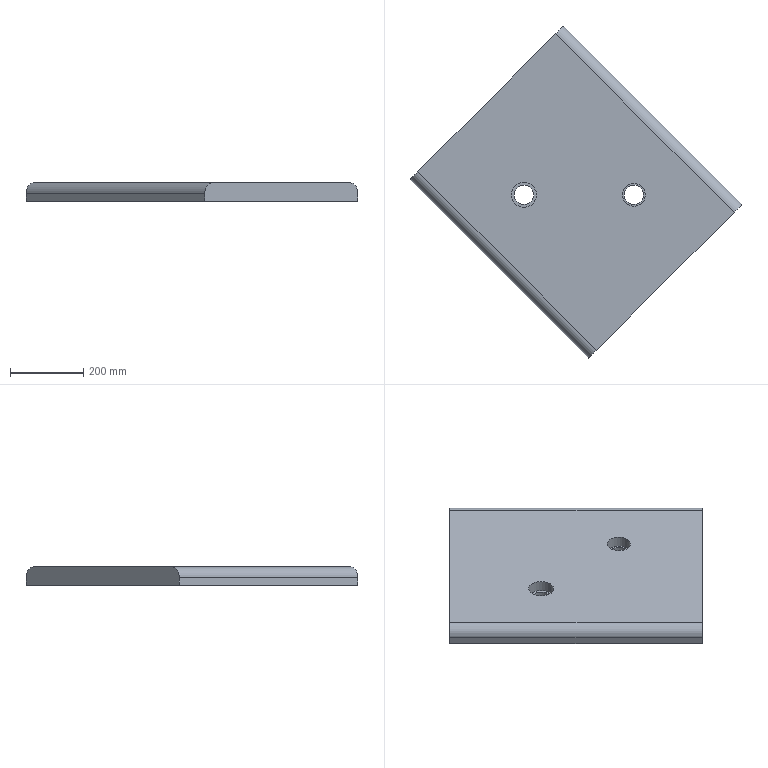Part | SolidWorks | 1 solid | 18 faces | box 906.604 x 906.604 x 50 mm | volume 19871305 mm3 | cylinder 10 | plane 8 | commonest cylinder face diameters 53 x4 60 x2 63 x2 68 x2
STEP:
#1=CARTESIAN_POINT('',(268.5,0.,35.));
#2=VERTEX_POINT('',#1);
#3=CARTESIAN_POINT('',(331.5,0.,35.));
#4=VERTEX_POINT('',#3);
#5=CARTESIAN_POINT('',(300.,0.,35.));
#6=DIRECTION('',(0.,0.,-1.));
#7=DIRECTION('',(-1.,0.,0.));
#8=AXIS2_PLACEMENT_3D('',#5,#6,#7);
#9=CIRCLE('',#8,31.5);
#10=EDGE_CURVE('',#2,#4,#9,.T.);
#11=ORIENTED_EDGE('',*,*,#10,.T.);
#12=CARTESIAN_POINT('',(331.5,0.,65.));
#13=VERTEX_POINT('',#12);
#14=CARTESIAN_POINT('',(331.5,0.,35.));
#15=DIRECTION('',(0.,0.,1.));
#16=VECTOR('',#15,1000.);
#17=LINE('',#14,#16);
#18=EDGE_CURVE('',#4,#13,#17,.T.);
#19=ORIENTED_EDGE('',*,*,#18,.T.);
#20=CARTESIAN_POINT('',(268.5,0.,65.));
#21=VERTEX_POINT('',#20);
#22=CARTESIAN_POINT('',(300.,0.,65.));
#23=DIRECTION('',(0.,0.,1.));
#24=DIRECTION('',(1.,0.,0.));
#25=AXIS2_PLACEMENT_3D('',#22,#23,#24);
#26=CIRCLE('',#25,31.5);
#27=EDGE_CURVE('',#13,#21,#26,.T.);
#28=ORIENTED_EDGE('',*,*,#27,.T.);
#29=CARTESIAN_POINT('',(268.5,0.,35.));
#30=DIRECTION('',(0.,0.,1.));
#31=VECTOR('',#30,1000.);
#32=LINE('',#29,#31);
#33=EDGE_CURVE('',#2,#21,#32,.T.);
#34=ORIENTED_EDGE('',*,*,#33,.F.);
#35=EDGE_LOOP('',(#11,#19,#28,#34));
#36=FACE_OUTER_BOUND('',#35,.T.);
#37=CARTESIAN_POINT('',(300.,0.,65.));
#38=DIRECTION('',(0.,0.,1.));
#39=DIRECTION('',(1.,0.,0.));
#40=AXIS2_PLACEMENT_3D('',#37,#38,#39);
#41=CYLINDRICAL_SURFACE('',#40,31.5);
#42=ADVANCED_FACE('',(#36),#41,.F.);
#43=CARTESIAN_POINT('',(300.,0.,35.));
#44=DIRECTION('',(0.,0.,-1.));
#45=DIRECTION('',(1.,0.,0.));
#46=AXIS2_PLACEMENT_3D('',#43,#44,#45);
#47=CIRCLE('',#46,31.5);
#48=EDGE_CURVE('',#4,#2,#47,.T.);
#49=ORIENTED_EDGE('',*,*,#48,.T.);
#50=ORIENTED_EDGE('',*,*,#33,.T.);
#51=CARTESIAN_POINT('',(300.,0.,65.));
#52=DIRECTION('',(0.,0.,1.));
#53=DIRECTION('',(-1.,0.,0.));
#54=AXIS2_PLACEMENT_3D('',#51,#52,#53);
#55=CIRCLE('',#54,31.5);
#56=EDGE_CURVE('',#21,#13,#55,.T.);
#57=ORIENTED_EDGE('',*,*,#56,.T.);
#58=ORIENTED_EDGE('',*,*,#18,.F.);
#59=EDGE_LOOP('',(#49,#50,#57,#58));
#60=FACE_OUTER_BOUND('',#59,.T.);
#61=CARTESIAN_POINT('',(300.,0.,65.));
#62=DIRECTION('',(0.,0.,1.));
#63=DIRECTION('',(1.,0.,0.));
#64=AXIS2_PLACEMENT_3D('',#61,#62,#63);
#65=CYLINDRICAL_SURFACE('',#64,31.5);
#66=ADVANCED_FACE('',(#60),#65,.F.);
#67=CARTESIAN_POINT('',(326.5,0.,35.));
#68=VERTEX_POINT('',#67);
#69=CARTESIAN_POINT('',(273.5,0.,35.));
#70=VERTEX_POINT('',#69);
#71=CARTESIAN_POINT('',(300.,0.,35.));
#72=DIRECTION('',(0.,0.,1.));
#73=DIRECTION('',(1.,0.,0.));
#74=AXIS2_PLACEMENT_3D('',#71,#72,#73);
#75=CIRCLE('',#74,26.5);
#76=EDGE_CURVE('',#68,#70,#75,.T.);
#77=ORIENTED_EDGE('',*,*,#76,.F.);
#78=CARTESIAN_POINT('',(300.,0.,35.));
#79=DIRECTION('',(0.,0.,1.));
#80=DIRECTION('',(-1.,0.,0.));
#81=AXIS2_PLACEMENT_3D('',#78,#79,#80);
#82=CIRCLE('',#81,26.5);
#83=EDGE_CURVE('',#70,#68,#82,.T.);
#84=ORIENTED_EDGE('',*,*,#83,.F.);
#85=EDGE_LOOP('',(#77,#84));
#86=FACE_BOUND('',#85,.T.);
#87=ORIENTED_EDGE('',*,*,#10,.F.);
#88=ORIENTED_EDGE('',*,*,#48,.F.);
#89=EDGE_LOOP('',(#87,#88));
#90=FACE_OUTER_BOUND('',#89,.T.);
#91=CARTESIAN_POINT('',(0.,0.,35.));
#92=DIRECTION('',(0.,0.,1.));
#93=DIRECTION('',(1.,0.,0.));
#94=AXIS2_PLACEMENT_3D('',#91,#92,#93);
#95=PLANE('',#94);
#96=ADVANCED_FACE('',(#86,#90),#95,.T.);
#97=CARTESIAN_POINT('',(273.5,0.,15.));
#98=VERTEX_POINT('',#97);
#99=CARTESIAN_POINT('',(326.5,0.,15.));
#100=VERTEX_POINT('',#99);
#101=CARTESIAN_POINT('',(300.,0.,15.));
#102=DIRECTION('',(0.,0.,-1.));
#103=DIRECTION('',(-1.,0.,0.));
#104=AXIS2_PLACEMENT_3D('',#101,#102,#103);
#105=CIRCLE('',#104,26.5);
#106=EDGE_CURVE('',#98,#100,#105,.T.);
#107=ORIENTED_EDGE('',*,*,#106,.T.);
#108=CARTESIAN_POINT('',(326.5,0.,15.));
#109=DIRECTION('',(0.,0.,1.));
#110=VECTOR('',#109,1000.);
#111=LINE('',#108,#110);
#112=EDGE_CURVE('',#100,#68,#111,.T.);
#113=ORIENTED_EDGE('',*,*,#112,.T.);
#114=ORIENTED_EDGE('',*,*,#76,.T.);
#115=CARTESIAN_POINT('',(273.5,0.,15.));
#116=DIRECTION('',(0.,0.,1.));
#117=VECTOR('',#116,1000.);
#118=LINE('',#115,#117);
#119=EDGE_CURVE('',#98,#70,#118,.T.);
#120=ORIENTED_EDGE('',*,*,#119,.F.);
#121=EDGE_LOOP('',(#107,#113,#114,#120));
#122=FACE_OUTER_BOUND('',#121,.T.);
#123=CARTESIAN_POINT('',(300.,0.,65.));
#124=DIRECTION('',(0.,0.,1.));
#125=DIRECTION('',(1.,0.,0.));
#126=AXIS2_PLACEMENT_3D('',#123,#124,#125);
#127=CYLINDRICAL_SURFACE('',#126,26.5);
#128=ADVANCED_FACE('',(#122),#127,.F.);
#129=CARTESIAN_POINT('',(300.,0.,15.));
#130=DIRECTION('',(0.,0.,-1.));
#131=DIRECTION('',(1.,0.,0.));
#132=AXIS2_PLACEMENT_3D('',#129,#130,#131);
#133=CIRCLE('',#132,26.5);
#134=EDGE_CURVE('',#100,#98,#133,.T.);
#135=ORIENTED_EDGE('',*,*,#134,.T.);
#136=ORIENTED_EDGE('',*,*,#119,.T.);
#137=ORIENTED_EDGE('',*,*,#83,.T.);
#138=ORIENTED_EDGE('',*,*,#112,.F.);
#139=EDGE_LOOP('',(#135,#136,#137,#138));
#140=FACE_OUTER_BOUND('',#139,.T.);
#141=CARTESIAN_POINT('',(300.,0.,65.));
#142=DIRECTION('',(0.,0.,1.));
#143=DIRECTION('',(1.,0.,0.));
#144=AXIS2_PLACEMENT_3D('',#141,#142,#143);
#145=CYLINDRICAL_SURFACE('',#144,26.5);
#146=ADVANCED_FACE('',(#140),#145,.F.);
#147=CARTESIAN_POINT('',(26.5,0.,35.));
#148=VERTEX_POINT('',#147);
#149=CARTESIAN_POINT('',(-26.5,0.,35.));
#150=VERTEX_POINT('',#149);
#151=CARTESIAN_POINT('',(0.,0.,35.));
#152=DIRECTION('',(0.,0.,1.));
#153=DIRECTION('',(1.,0.,0.));
#154=AXIS2_PLACEMENT_3D('',#151,#152,#153);
#155=CIRCLE('',#154,26.5);
#156=EDGE_CURVE('',#148,#150,#155,.T.);
#157=ORIENTED_EDGE('',*,*,#156,.F.);
#158=CARTESIAN_POINT('',(0.,0.,35.));
#159=DIRECTION('',(0.,0.,1.));
#160=DIRECTION('',(-1.,0.,0.));
#161=AXIS2_PLACEMENT_3D('',#158,#159,#160);
#162=CIRCLE('',#161,26.5);
#163=EDGE_CURVE('',#150,#148,#162,.T.);
#164=ORIENTED_EDGE('',*,*,#163,.F.);
#165=EDGE_LOOP('',(#157,#164));
#166=FACE_BOUND('',#165,.T.);
#167=CARTESIAN_POINT('',(-34.,0.,35.));
#168=VERTEX_POINT('',#167);
#169=CARTESIAN_POINT('',(34.,0.,35.));
#170=VERTEX_POINT('',#169);
#171=CARTESIAN_POINT('',(0.,0.,35.));
#172=DIRECTION('',(0.,0.,-1.));
#173=DIRECTION('',(-1.,0.,0.));
#174=AXIS2_PLACEMENT_3D('',#171,#172,#173);
#175=CIRCLE('',#174,34.);
#176=EDGE_CURVE('',#168,#170,#175,.T.);
#177=ORIENTED_EDGE('',*,*,#176,.F.);
#178=CARTESIAN_POINT('',(0.,0.,35.));
#179=DIRECTION('',(0.,0.,-1.));
#180=DIRECTION('',(1.,0.,0.));
#181=AXIS2_PLACEMENT_3D('',#178,#179,#180);
#182=CIRCLE('',#181,34.);
#183=EDGE_CURVE('',#170,#168,#182,.T.);
#184=ORIENTED_EDGE('',*,*,#183,.F.);
#185=EDGE_LOOP('',(#177,#184));
#186=FACE_OUTER_BOUND('',#185,.T.);
#187=CARTESIAN_POINT('',(0.,0.,35.));
#188=DIRECTION('',(0.,0.,1.));
#189=DIRECTION('',(1.,0.,0.));
#190=AXIS2_PLACEMENT_3D('',#187,#188,#189);
#191=PLANE('',#190);
#192=ADVANCED_FACE('',(#166,#186),#191,.T.);
#193=CARTESIAN_POINT('',(-26.5,0.,15.));
#194=VERTEX_POINT('',#193);
#195=CARTESIAN_POINT('',(26.5,0.,15.));
#196=VERTEX_POINT('',#195);
#197=CARTESIAN_POINT('',(0.,0.,15.));
#198=DIRECTION('',(0.,0.,-1.));
#199=DIRECTION('',(-1.,0.,0.));
#200=AXIS2_PLACEMENT_3D('',#197,#198,#199);
#201=CIRCLE('',#200,26.5);
#202=EDGE_CURVE('',#194,#196,#201,.T.);
#203=ORIENTED_EDGE('',*,*,#202,.T.);
#204=CARTESIAN_POINT('',(26.5,0.,15.));
#205=DIRECTION('',(0.,0.,1.));
#206=VECTOR('',#205,1000.);
#207=LINE('',#204,#206);
#208=EDGE_CURVE('',#196,#148,#207,.T.);
#209=ORIENTED_EDGE('',*,*,#208,.T.);
#210=ORIENTED_EDGE('',*,*,#156,.T.);
#211=CARTESIAN_POINT('',(-26.5,0.,15.));
#212=DIRECTION('',(0.,0.,1.));
#213=VECTOR('',#212,1000.);
#214=LINE('',#211,#213);
#215=EDGE_CURVE('',#194,#150,#214,.T.);
#216=ORIENTED_EDGE('',*,*,#215,.F.);
#217=EDGE_LOOP('',(#203,#209,#210,#216));
#218=FACE_OUTER_BOUND('',#217,.T.);
#219=CARTESIAN_POINT('',(0.,0.,65.));
#220=DIRECTION('',(0.,0.,1.));
#221=DIRECTION('',(1.,0.,0.));
#222=AXIS2_PLACEMENT_3D('',#219,#220,#221);
#223=CYLINDRICAL_SURFACE('',#222,26.5);
#224=ADVANCED_FACE('',(#218),#223,.F.);
#225=CARTESIAN_POINT('',(0.,0.,15.));
#226=DIRECTION('',(0.,0.,-1.));
#227=DIRECTION('',(1.,0.,0.));
#228=AXIS2_PLACEMENT_3D('',#225,#226,#227);
#229=CIRCLE('',#228,26.5);
#230=EDGE_CURVE('',#196,#194,#229,.T.);
#231=ORIENTED_EDGE('',*,*,#230,.T.);
#232=ORIENTED_EDGE('',*,*,#215,.T.);
#233=ORIENTED_EDGE('',*,*,#163,.T.);
#234=ORIENTED_EDGE('',*,*,#208,.F.);
#235=EDGE_LOOP('',(#231,#232,#233,#234));
#236=FACE_OUTER_BOUND('',#235,.T.);
#237=CARTESIAN_POINT('',(0.,0.,65.));
#238=DIRECTION('',(0.,0.,1.));
#239=DIRECTION('',(1.,0.,0.));
#240=AXIS2_PLACEMENT_3D('',#237,#238,#239);
#241=CYLINDRICAL_SURFACE('',#240,26.5);
#242=ADVANCED_FACE('',(#236),#241,.F.);
#243=ORIENTED_EDGE('',*,*,#106,.F.);
#244=ORIENTED_EDGE('',*,*,#134,.F.);
#245=EDGE_LOOP('',(#243,#244));
#246=FACE_BOUND('',#245,.T.);
#247=ORIENTED_EDGE('',*,*,#202,.F.);
#248=ORIENTED_EDGE('',*,*,#230,.F.);
#249=EDGE_LOOP('',(#247,#248));
#250=FACE_BOUND('',#249,.T.);
#251=CARTESIAN_POINT('',(595.477,-26.777,15.));
#252=VERTEX_POINT('',#251);
#253=CARTESIAN_POINT('',(107.574,461.127,15.));
#254=VERTEX_POINT('',#253);
#255=CARTESIAN_POINT('',(595.477,-26.777,15.));
#256=DIRECTION('',(-0.7071,0.7071,0.));
#257=VECTOR('',#256,1000.);
#258=LINE('',#255,#257);
#259=EDGE_CURVE('',#252,#254,#258,.T.);
#260=ORIENTED_EDGE('',*,*,#259,.F.);
#261=CARTESIAN_POINT('',(176.777,-445.477,15.));
#262=VERTEX_POINT('',#261);
#263=CARTESIAN_POINT('',(176.777,-445.477,15.));
#264=DIRECTION('',(0.7071,0.7071,0.));
#265=VECTOR('',#264,1000.);
#266=LINE('',#263,#265);
#267=EDGE_CURVE('',#262,#252,#266,.T.);
#268=ORIENTED_EDGE('',*,*,#267,.F.);
#269=CARTESIAN_POINT('',(-311.127,42.426,15.));
#270=VERTEX_POINT('',#269);
#271=CARTESIAN_POINT('',(-311.127,42.426,15.));
#272=DIRECTION('',(0.7071,-0.7071,0.));
#273=VECTOR('',#272,1000.);
#274=LINE('',#271,#273);
#275=EDGE_CURVE('',#270,#262,#274,.T.);
#276=ORIENTED_EDGE('',*,*,#275,.F.);
#277=CARTESIAN_POINT('',(107.574,461.127,15.));
#278=DIRECTION('',(-0.7071,-0.7071,0.));
#279=VECTOR('',#278,1000.);
#280=LINE('',#277,#279);
#281=EDGE_CURVE('',#254,#270,#280,.T.);
#282=ORIENTED_EDGE('',*,*,#281,.F.);
#283=EDGE_LOOP('',(#260,#268,#276,#282));
#284=FACE_OUTER_BOUND('',#283,.T.);
#285=CARTESIAN_POINT('',(0.,0.,15.));
#286=DIRECTION('',(0.,0.,1.));
#287=DIRECTION('',(1.,0.,0.));
#288=AXIS2_PLACEMENT_3D('',#285,#286,#287);
#289=PLANE('',#288);
#290=ADVANCED_FACE('',(#246,#250,#284),#289,.F.);
#291=CARTESIAN_POINT('',(176.777,-445.477,35.));
#292=VERTEX_POINT('',#291);
#293=CARTESIAN_POINT('',(176.777,-445.477,65.));
#294=DIRECTION('',(0.,0.,-1.));
#295=VECTOR('',#294,1000.);
#296=LINE('',#293,#295);
#297=EDGE_CURVE('',#292,#262,#296,.T.);
#298=ORIENTED_EDGE('',*,*,#297,.F.);
#299=CARTESIAN_POINT('',(-311.127,42.426,35.));
#300=VERTEX_POINT('',#299);
#301=CARTESIAN_POINT('',(-311.127,42.426,35.));
#302=DIRECTION('',(-0.7071,0.7071,0.));
#303=VECTOR('',#302,1000.);
#304=LINE('',#301,#303);
#305=EDGE_CURVE('',#292,#300,#304,.T.);
#306=ORIENTED_EDGE('',*,*,#305,.T.);
#307=CARTESIAN_POINT('',(-311.127,42.426,65.));
#308=DIRECTION('',(0.,0.,-1.));
#309=VECTOR('',#308,1000.);
#310=LINE('',#307,#309);
#311=EDGE_CURVE('',#300,#270,#310,.T.);
#312=ORIENTED_EDGE('',*,*,#311,.T.);
#313=ORIENTED_EDGE('',*,*,#275,.T.);
#314=EDGE_LOOP('',(#298,#306,#312,#313));
#315=FACE_OUTER_BOUND('',#314,.T.);
#316=CARTESIAN_POINT('',(-311.127,42.426,15.));
#317=DIRECTION('',(-0.7071,-0.7071,0.));
#318=DIRECTION('',(-0.7071,0.7071,0.));
#319=AXIS2_PLACEMENT_3D('',#316,#317,#318);
#320=PLANE('',#319);
#321=ADVANCED_FACE('',(#315),#320,.T.);
#322=ORIENTED_EDGE('',*,*,#311,.F.);
#323=CARTESIAN_POINT('',(-289.914,63.64,65.));
#324=VERTEX_POINT('',#323);
#325=CARTESIAN_POINT('',(-289.914,63.64,35.));
#326=DIRECTION('',(-0.7071,0.7071,0.));
#327=DIRECTION('',(-0.7071,-0.7071,0.));
#328=AXIS2_PLACEMENT_3D('',#325,#326,#327);
#329=CIRCLE('',#328,30.);
#330=EDGE_CURVE('',#300,#324,#329,.T.);
#331=ORIENTED_EDGE('',*,*,#330,.T.);
#332=CARTESIAN_POINT('',(86.36,439.914,65.));
#333=VERTEX_POINT('',#332);
#334=CARTESIAN_POINT('',(-311.127,42.426,65.));
#335=DIRECTION('',(0.7071,0.7071,0.));
#336=VECTOR('',#335,1000.);
#337=LINE('',#334,#336);
#338=EDGE_CURVE('',#324,#333,#337,.T.);
#339=ORIENTED_EDGE('',*,*,#338,.T.);
#340=CARTESIAN_POINT('',(107.574,461.127,35.));
#341=VERTEX_POINT('',#340);
#342=CARTESIAN_POINT('',(86.36,439.914,35.));
#343=DIRECTION('',(-0.7071,0.7071,0.));
#344=DIRECTION('',(-0.7071,-0.7071,0.));
#345=AXIS2_PLACEMENT_3D('',#342,#343,#344);
#346=CIRCLE('',#345,30.);
#347=EDGE_CURVE('',#333,#341,#346,.T.);
#348=ORIENTED_EDGE('',*,*,#347,.T.);
#349=CARTESIAN_POINT('',(107.574,461.127,65.));
#350=DIRECTION('',(0.,0.,-1.));
#351=VECTOR('',#350,1000.);
#352=LINE('',#349,#351);
#353=EDGE_CURVE('',#341,#254,#352,.T.);
#354=ORIENTED_EDGE('',*,*,#353,.T.);
#355=ORIENTED_EDGE('',*,*,#281,.T.);
#356=EDGE_LOOP('',(#322,#331,#339,#348,#354,#355));
#357=FACE_OUTER_BOUND('',#356,.T.);
#358=CARTESIAN_POINT('',(107.574,461.127,15.));
#359=DIRECTION('',(-0.7071,0.7071,0.));
#360=DIRECTION('',(0.,0.,1.));
#361=AXIS2_PLACEMENT_3D('',#358,#359,#360);
#362=PLANE('',#361);
#363=ADVANCED_FACE('',(#357),#362,.T.);
#364=ORIENTED_EDGE('',*,*,#353,.F.);
#365=CARTESIAN_POINT('',(595.477,-26.777,35.));
#366=VERTEX_POINT('',#365);
#367=CARTESIAN_POINT('',(595.477,-26.777,35.));
#368=DIRECTION('',(0.7071,-0.7071,0.));
#369=VECTOR('',#368,1000.);
#370=LINE('',#367,#369);
#371=EDGE_CURVE('',#341,#366,#370,.T.);
#372=ORIENTED_EDGE('',*,*,#371,.T.);
#373=CARTESIAN_POINT('',(595.477,-26.777,65.));
#374=DIRECTION('',(0.,0.,-1.));
#375=VECTOR('',#374,1000.);
#376=LINE('',#373,#375);
#377=EDGE_CURVE('',#366,#252,#376,.T.);
#378=ORIENTED_EDGE('',*,*,#377,.T.);
#379=ORIENTED_EDGE('',*,*,#259,.T.);
#380=EDGE_LOOP('',(#364,#372,#378,#379));
#381=FACE_OUTER_BOUND('',#380,.T.);
#382=CARTESIAN_POINT('',(595.477,-26.777,15.));
#383=DIRECTION('',(0.7071,0.7071,0.));
#384=DIRECTION('',(0.,0.,-1.));
#385=AXIS2_PLACEMENT_3D('',#382,#383,#384);
#386=PLANE('',#385);
#387=ADVANCED_FACE('',(#381),#386,.T.);
#388=CARTESIAN_POINT('',(574.264,-47.99,65.));
#389=VERTEX_POINT('',#388);
#390=CARTESIAN_POINT('',(197.99,-424.264,65.));
#391=VERTEX_POINT('',#390);
#392=CARTESIAN_POINT('',(595.477,-26.777,65.));
#393=DIRECTION('',(-0.7071,-0.7071,0.));
#394=VECTOR('',#393,1000.);
#395=LINE('',#392,#394);
#396=EDGE_CURVE('',#389,#391,#395,.T.);
#397=ORIENTED_EDGE('',*,*,#396,.T.);
#398=CARTESIAN_POINT('',(197.99,-424.264,35.));
#399=DIRECTION('',(0.7071,-0.7071,0.));
#400=DIRECTION('',(0.7071,0.7071,0.));
#401=AXIS2_PLACEMENT_3D('',#398,#399,#400);
#402=CIRCLE('',#401,30.);
#403=EDGE_CURVE('',#391,#292,#402,.T.);
#404=ORIENTED_EDGE('',*,*,#403,.T.);
#405=ORIENTED_EDGE('',*,*,#297,.T.);
#406=ORIENTED_EDGE('',*,*,#267,.T.);
#407=ORIENTED_EDGE('',*,*,#377,.F.);
#408=CARTESIAN_POINT('',(574.264,-47.99,35.));
#409=DIRECTION('',(0.7071,-0.7071,0.));
#410=DIRECTION('',(0.7071,0.7071,0.));
#411=AXIS2_PLACEMENT_3D('',#408,#409,#410);
#412=CIRCLE('',#411,30.);
#413=EDGE_CURVE('',#366,#389,#412,.T.);
#414=ORIENTED_EDGE('',*,*,#413,.T.);
#415=EDGE_LOOP('',(#397,#404,#405,#406,#407,#414));
#416=FACE_OUTER_BOUND('',#415,.T.);
#417=CARTESIAN_POINT('',(176.777,-445.477,15.));
#418=DIRECTION('',(0.7071,-0.7071,0.));
#419=DIRECTION('',(0.,0.,-1.));
#420=AXIS2_PLACEMENT_3D('',#417,#418,#419);
#421=PLANE('',#420);
#422=ADVANCED_FACE('',(#416),#421,.T.);
#423=ORIENTED_EDGE('',*,*,#27,.F.);
#424=ORIENTED_EDGE('',*,*,#56,.F.);
#425=EDGE_LOOP('',(#423,#424));
#426=FACE_BOUND('',#425,.T.);
#427=CARTESIAN_POINT('',(34.,0.,65.));
#428=VERTEX_POINT('',#427);
#429=CARTESIAN_POINT('',(-34.,0.,65.));
#430=VERTEX_POINT('',#429);
#431=CARTESIAN_POINT('',(0.,0.,65.));
#432=DIRECTION('',(0.,0.,1.));
#433=DIRECTION('',(1.,0.,0.));
#434=AXIS2_PLACEMENT_3D('',#431,#432,#433);
#435=CIRCLE('',#434,34.);
#436=EDGE_CURVE('',#428,#430,#435,.T.);
#437=ORIENTED_EDGE('',*,*,#436,.F.);
#438=CARTESIAN_POINT('',(0.,0.,65.));
#439=DIRECTION('',(0.,0.,1.));
#440=DIRECTION('',(-1.,0.,0.));
#441=AXIS2_PLACEMENT_3D('',#438,#439,#440);
#442=CIRCLE('',#441,34.);
#443=EDGE_CURVE('',#430,#428,#442,.T.);
#444=ORIENTED_EDGE('',*,*,#443,.F.);
#445=EDGE_LOOP('',(#437,#444));
#446=FACE_BOUND('',#445,.T.);
#447=ORIENTED_EDGE('',*,*,#338,.F.);
#448=CARTESIAN_POINT('',(-113.137,-113.137,65.));
#449=DIRECTION('',(0.7071,-0.7071,0.));
#450=VECTOR('',#449,1000.);
#451=LINE('',#448,#450);
#452=EDGE_CURVE('',#324,#391,#451,.T.);
#453=ORIENTED_EDGE('',*,*,#452,.T.);
#454=ORIENTED_EDGE('',*,*,#396,.F.);
#455=CARTESIAN_POINT('',(263.137,263.137,65.));
#456=DIRECTION('',(-0.7071,0.7071,0.));
#457=VECTOR('',#456,1000.);
#458=LINE('',#455,#457);
#459=EDGE_CURVE('',#389,#333,#458,.T.);
#460=ORIENTED_EDGE('',*,*,#459,.T.);
#461=EDGE_LOOP('',(#447,#453,#454,#460));
#462=FACE_OUTER_BOUND('',#461,.T.);
#463=CARTESIAN_POINT('',(0.,0.,65.));
#464=DIRECTION('',(0.,0.,1.));
#465=DIRECTION('',(1.,0.,0.));
#466=AXIS2_PLACEMENT_3D('',#463,#464,#465);
#467=PLANE('',#466);
#468=ADVANCED_FACE('',(#426,#446,#462),#467,.T.);
#469=ORIENTED_EDGE('',*,*,#183,.T.);
#470=CARTESIAN_POINT('',(-34.,0.,35.));
#471=DIRECTION('',(0.,0.,1.));
#472=VECTOR('',#471,1000.);
#473=LINE('',#470,#472);
#474=EDGE_CURVE('',#168,#430,#473,.T.);
#475=ORIENTED_EDGE('',*,*,#474,.T.);
#476=ORIENTED_EDGE('',*,*,#443,.T.);
#477=CARTESIAN_POINT('',(34.,0.,35.));
#478=DIRECTION('',(0.,0.,1.));
#479=VECTOR('',#478,1000.);
#480=LINE('',#477,#479);
#481=EDGE_CURVE('',#170,#428,#480,.T.);
#482=ORIENTED_EDGE('',*,*,#481,.F.);
#483=EDGE_LOOP('',(#469,#475,#476,#482));
#484=FACE_OUTER_BOUND('',#483,.T.);
#485=CARTESIAN_POINT('',(0.,0.,65.));
#486=DIRECTION('',(0.,0.,1.));
#487=DIRECTION('',(1.,0.,0.));
#488=AXIS2_PLACEMENT_3D('',#485,#486,#487);
#489=CYLINDRICAL_SURFACE('',#488,34.);
#490=ADVANCED_FACE('',(#484),#489,.F.);
#491=ORIENTED_EDGE('',*,*,#176,.T.);
#492=ORIENTED_EDGE('',*,*,#481,.T.);
#493=ORIENTED_EDGE('',*,*,#436,.T.);
#494=ORIENTED_EDGE('',*,*,#474,.F.);
#495=EDGE_LOOP('',(#491,#492,#493,#494));
#496=FACE_OUTER_BOUND('',#495,.T.);
#497=CARTESIAN_POINT('',(0.,0.,65.));
#498=DIRECTION('',(0.,0.,1.));
#499=DIRECTION('',(1.,0.,0.));
#500=AXIS2_PLACEMENT_3D('',#497,#498,#499);
#501=CYLINDRICAL_SURFACE('',#500,34.);
#502=ADVANCED_FACE('',(#496),#501,.F.);
#503=ORIENTED_EDGE('',*,*,#403,.F.);
#504=ORIENTED_EDGE('',*,*,#452,.F.);
#505=ORIENTED_EDGE('',*,*,#330,.F.);
#506=ORIENTED_EDGE('',*,*,#305,.F.);
#507=EDGE_LOOP('',(#503,#504,#505,#506));
#508=FACE_OUTER_BOUND('',#507,.T.);
#509=CARTESIAN_POINT('',(-289.914,63.64,35.));
#510=DIRECTION('',(-0.7071,0.7071,0.));
#511=DIRECTION('',(-0.7071,-0.7071,0.));
#512=AXIS2_PLACEMENT_3D('',#509,#510,#511);
#513=CYLINDRICAL_SURFACE('',#512,30.);
#514=ADVANCED_FACE('',(#508),#513,.T.);
#515=ORIENTED_EDGE('',*,*,#347,.F.);
#516=ORIENTED_EDGE('',*,*,#459,.F.);
#517=ORIENTED_EDGE('',*,*,#413,.F.);
#518=ORIENTED_EDGE('',*,*,#371,.F.);
#519=EDGE_LOOP('',(#515,#516,#517,#518));
#520=FACE_OUTER_BOUND('',#519,.T.);
#521=CARTESIAN_POINT('',(574.264,-47.99,35.));
#522=DIRECTION('',(0.7071,-0.7071,0.));
#523=DIRECTION('',(0.7071,0.7071,0.));
#524=AXIS2_PLACEMENT_3D('',#521,#522,#523);
#525=CYLINDRICAL_SURFACE('',#524,30.);
#526=ADVANCED_FACE('',(#520),#525,.T.);
#527=CLOSED_SHELL('',(#42,#66,#96,#128,#146,#192,#224,#242,#290,#321,#363,#387,#422,#468,#490,#502,#514,#526));
#528=MANIFOLD_SOLID_BREP('',#527);
#529=CARTESIAN_POINT('',(0.,0.,0.));
#530=DIRECTION('',(0.,0.,1.));
#531=DIRECTION('',(1.,0.,0.));
#532=AXIS2_PLACEMENT_3D('',#529,#530,#531);
#533=(LENGTH_UNIT()NAMED_UNIT(*)SI_UNIT(.MILLI.,.METRE.));
#534=UNCERTAINTY_MEASURE_WITH_UNIT(LENGTH_MEASURE(0.00001),#533,'','');
#535=(NAMED_UNIT(*)PLANE_ANGLE_UNIT()SI_UNIT($,.RADIAN.));
#536=(NAMED_UNIT(*)SI_UNIT($,.STERADIAN.)SOLID_ANGLE_UNIT());
#537=(GEOMETRIC_REPRESENTATION_CONTEXT(3)GLOBAL_UNCERTAINTY_ASSIGNED_CONTEXT((#534))GLOBAL_UNIT_ASSIGNED_CONTEXT((#533,#535,#536))REPRESENTATION_CONTEXT('',''));
#538=ADVANCED_BREP_SHAPE_REPRESENTATION('',(#528,#532),#537);